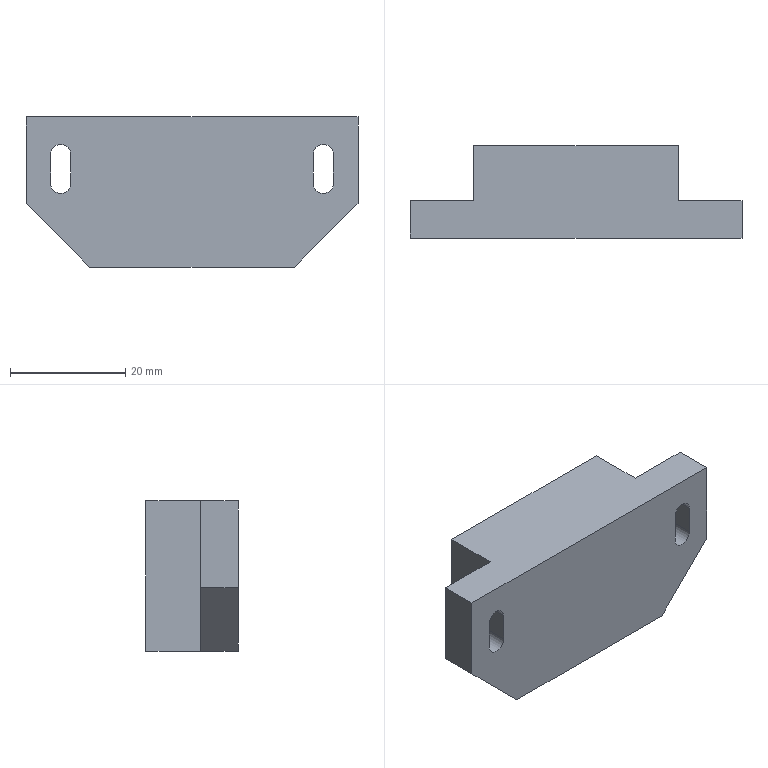Part | STEP file | Large white magnetic mount | 1 solid | 20 faces | box 57.5 x 16 x 26 mm | volume 17347 mm3 | plane 16 | cylinder 4 | commonest cylinder face diameters 3.5 x4
STEP:
#1=CARTESIAN_POINT('',(4.25,6.5,-6.5));
#2=VERTEX_POINT('',#1);
#3=CARTESIAN_POINT('',(7.75,6.5,-6.5));
#4=VERTEX_POINT('',#3);
#5=CARTESIAN_POINT('',(6.,6.5,-6.5));
#6=DIRECTION('',(0.,1.,0.));
#7=DIRECTION('',(0.,0.,1.));
#8=AXIS2_PLACEMENT_3D('',#5,#6,#7);
#9=CIRCLE('',#8,1.75);
#10=EDGE_CURVE('',#2,#4,#9,.T.);
#11=ORIENTED_EDGE('',*,*,#10,.F.);
#12=CARTESIAN_POINT('',(4.25,6.5,-11.5));
#13=VERTEX_POINT('',#12);
#14=CARTESIAN_POINT('',(4.25,6.5,-6.5));
#15=DIRECTION('',(0.,0.,1.));
#16=VECTOR('',#15,1000.);
#17=LINE('',#14,#16);
#18=EDGE_CURVE('',#13,#2,#17,.T.);
#19=ORIENTED_EDGE('',*,*,#18,.F.);
#20=CARTESIAN_POINT('',(7.75,6.5,-11.5));
#21=VERTEX_POINT('',#20);
#22=CARTESIAN_POINT('',(6.,6.5,-11.5));
#23=DIRECTION('',(0.,1.,0.));
#24=DIRECTION('',(0.,0.,1.));
#25=AXIS2_PLACEMENT_3D('',#22,#23,#24);
#26=CIRCLE('',#25,1.75);
#27=EDGE_CURVE('',#21,#13,#26,.T.);
#28=ORIENTED_EDGE('',*,*,#27,.F.);
#29=CARTESIAN_POINT('',(7.75,6.5,-6.5));
#30=DIRECTION('',(0.,0.,-1.));
#31=VECTOR('',#30,1000.);
#32=LINE('',#29,#31);
#33=EDGE_CURVE('',#4,#21,#32,.T.);
#34=ORIENTED_EDGE('',*,*,#33,.F.);
#35=EDGE_LOOP('',(#11,#19,#28,#34));
#36=FACE_BOUND('',#35,.T.);
#37=CARTESIAN_POINT('',(11.,6.5,-26.));
#38=VERTEX_POINT('',#37);
#39=CARTESIAN_POINT('',(11.,6.5,0.));
#40=VERTEX_POINT('',#39);
#41=CARTESIAN_POINT('',(11.,6.5,-26.));
#42=DIRECTION('',(0.,0.,1.));
#43=VECTOR('',#42,1000.);
#44=LINE('',#41,#43);
#45=EDGE_CURVE('',#38,#40,#44,.T.);
#46=ORIENTED_EDGE('',*,*,#45,.F.);
#47=CARTESIAN_POINT('',(0.,6.5,-15.));
#48=VERTEX_POINT('',#47);
#49=CARTESIAN_POINT('',(0.,6.5,-15.));
#50=DIRECTION('',(-0.7071,0.,0.7071));
#51=VECTOR('',#50,1000.);
#52=LINE('',#49,#51);
#53=EDGE_CURVE('',#38,#48,#52,.T.);
#54=ORIENTED_EDGE('',*,*,#53,.T.);
#55=CARTESIAN_POINT('',(0.,6.5,0.));
#56=VERTEX_POINT('',#55);
#57=CARTESIAN_POINT('',(0.,6.5,0.));
#58=DIRECTION('',(0.,0.,1.));
#59=VECTOR('',#58,1000.);
#60=LINE('',#57,#59);
#61=EDGE_CURVE('',#48,#56,#60,.T.);
#62=ORIENTED_EDGE('',*,*,#61,.T.);
#63=CARTESIAN_POINT('',(57.5,6.5,0.));
#64=DIRECTION('',(1.,0.,0.));
#65=VECTOR('',#64,1000.);
#66=LINE('',#63,#65);
#67=EDGE_CURVE('',#56,#40,#66,.T.);
#68=ORIENTED_EDGE('',*,*,#67,.T.);
#69=EDGE_LOOP('',(#46,#54,#62,#68));
#70=FACE_OUTER_BOUND('',#69,.T.);
#71=CARTESIAN_POINT('',(0.,6.5,0.));
#72=DIRECTION('',(0.,-1.,0.));
#73=DIRECTION('',(0.,0.,-1.));
#74=AXIS2_PLACEMENT_3D('',#71,#72,#73);
#75=PLANE('',#74);
#76=ADVANCED_FACE('',(#36,#70),#75,.F.);
#77=CARTESIAN_POINT('',(49.75,6.5,-6.5));
#78=VERTEX_POINT('',#77);
#79=CARTESIAN_POINT('',(53.25,6.5,-6.5));
#80=VERTEX_POINT('',#79);
#81=CARTESIAN_POINT('',(51.5,6.5,-6.5));
#82=DIRECTION('',(0.,1.,0.));
#83=DIRECTION('',(0.,0.,-1.));
#84=AXIS2_PLACEMENT_3D('',#81,#82,#83);
#85=CIRCLE('',#84,1.75);
#86=EDGE_CURVE('',#78,#80,#85,.T.);
#87=ORIENTED_EDGE('',*,*,#86,.F.);
#88=CARTESIAN_POINT('',(49.75,6.5,-11.5));
#89=VERTEX_POINT('',#88);
#90=CARTESIAN_POINT('',(49.75,6.5,-6.5));
#91=DIRECTION('',(0.,0.,1.));
#92=VECTOR('',#91,1000.);
#93=LINE('',#90,#92);
#94=EDGE_CURVE('',#89,#78,#93,.T.);
#95=ORIENTED_EDGE('',*,*,#94,.F.);
#96=CARTESIAN_POINT('',(53.25,6.5,-11.5));
#97=VERTEX_POINT('',#96);
#98=CARTESIAN_POINT('',(51.5,6.5,-11.5));
#99=DIRECTION('',(0.,1.,0.));
#100=DIRECTION('',(0.,0.,-1.));
#101=AXIS2_PLACEMENT_3D('',#98,#99,#100);
#102=CIRCLE('',#101,1.75);
#103=EDGE_CURVE('',#97,#89,#102,.T.);
#104=ORIENTED_EDGE('',*,*,#103,.F.);
#105=CARTESIAN_POINT('',(53.25,6.5,-6.5));
#106=DIRECTION('',(0.,0.,-1.));
#107=VECTOR('',#106,1000.);
#108=LINE('',#105,#107);
#109=EDGE_CURVE('',#80,#97,#108,.T.);
#110=ORIENTED_EDGE('',*,*,#109,.F.);
#111=EDGE_LOOP('',(#87,#95,#104,#110));
#112=FACE_BOUND('',#111,.T.);
#113=CARTESIAN_POINT('',(46.5,6.5,0.));
#114=VERTEX_POINT('',#113);
#115=CARTESIAN_POINT('',(46.5,6.5,-26.));
#116=VERTEX_POINT('',#115);
#117=CARTESIAN_POINT('',(46.5,6.5,-26.));
#118=DIRECTION('',(0.,0.,-1.));
#119=VECTOR('',#118,1000.);
#120=LINE('',#117,#119);
#121=EDGE_CURVE('',#114,#116,#120,.T.);
#122=ORIENTED_EDGE('',*,*,#121,.F.);
#123=CARTESIAN_POINT('',(57.5,6.5,0.));
#124=VERTEX_POINT('',#123);
#125=CARTESIAN_POINT('',(57.5,6.5,0.));
#126=DIRECTION('',(1.,0.,0.));
#127=VECTOR('',#126,1000.);
#128=LINE('',#125,#127);
#129=EDGE_CURVE('',#114,#124,#128,.T.);
#130=ORIENTED_EDGE('',*,*,#129,.T.);
#131=CARTESIAN_POINT('',(57.5,6.5,-15.));
#132=VERTEX_POINT('',#131);
#133=CARTESIAN_POINT('',(57.5,6.5,-15.));
#134=DIRECTION('',(0.,0.,-1.));
#135=VECTOR('',#134,1000.);
#136=LINE('',#133,#135);
#137=EDGE_CURVE('',#124,#132,#136,.T.);
#138=ORIENTED_EDGE('',*,*,#137,.T.);
#139=CARTESIAN_POINT('',(46.5,6.5,-26.));
#140=DIRECTION('',(-0.7071,0.,-0.7071));
#141=VECTOR('',#140,1000.);
#142=LINE('',#139,#141);
#143=EDGE_CURVE('',#132,#116,#142,.T.);
#144=ORIENTED_EDGE('',*,*,#143,.T.);
#145=EDGE_LOOP('',(#122,#130,#138,#144));
#146=FACE_OUTER_BOUND('',#145,.T.);
#147=CARTESIAN_POINT('',(0.,6.5,0.));
#148=DIRECTION('',(0.,-1.,0.));
#149=DIRECTION('',(0.,0.,-1.));
#150=AXIS2_PLACEMENT_3D('',#147,#148,#149);
#151=PLANE('',#150);
#152=ADVANCED_FACE('',(#112,#146),#151,.F.);
#153=CARTESIAN_POINT('',(0.,0.,0.));
#154=VERTEX_POINT('',#153);
#155=CARTESIAN_POINT('',(57.5,0.,0.));
#156=VERTEX_POINT('',#155);
#157=CARTESIAN_POINT('',(57.5,0.,0.));
#158=DIRECTION('',(1.,0.,0.));
#159=VECTOR('',#158,1000.);
#160=LINE('',#157,#159);
#161=EDGE_CURVE('',#154,#156,#160,.T.);
#162=ORIENTED_EDGE('',*,*,#161,.F.);
#163=CARTESIAN_POINT('',(0.,0.,-15.));
#164=VERTEX_POINT('',#163);
#165=CARTESIAN_POINT('',(0.,0.,0.));
#166=DIRECTION('',(0.,0.,1.));
#167=VECTOR('',#166,1000.);
#168=LINE('',#165,#167);
#169=EDGE_CURVE('',#164,#154,#168,.T.);
#170=ORIENTED_EDGE('',*,*,#169,.F.);
#171=CARTESIAN_POINT('',(11.,0.,-26.));
#172=VERTEX_POINT('',#171);
#173=CARTESIAN_POINT('',(0.,0.,-15.));
#174=DIRECTION('',(-0.7071,0.,0.7071));
#175=VECTOR('',#174,1000.);
#176=LINE('',#173,#175);
#177=EDGE_CURVE('',#172,#164,#176,.T.);
#178=ORIENTED_EDGE('',*,*,#177,.F.);
#179=CARTESIAN_POINT('',(46.5,0.,-26.));
#180=VERTEX_POINT('',#179);
#181=CARTESIAN_POINT('',(11.,0.,-26.));
#182=DIRECTION('',(-1.,0.,0.));
#183=VECTOR('',#182,1000.);
#184=LINE('',#181,#183);
#185=EDGE_CURVE('',#180,#172,#184,.T.);
#186=ORIENTED_EDGE('',*,*,#185,.F.);
#187=CARTESIAN_POINT('',(57.5,0.,-15.));
#188=VERTEX_POINT('',#187);
#189=CARTESIAN_POINT('',(46.5,0.,-26.));
#190=DIRECTION('',(-0.7071,0.,-0.7071));
#191=VECTOR('',#190,1000.);
#192=LINE('',#189,#191);
#193=EDGE_CURVE('',#188,#180,#192,.T.);
#194=ORIENTED_EDGE('',*,*,#193,.F.);
#195=CARTESIAN_POINT('',(57.5,0.,-15.));
#196=DIRECTION('',(0.,0.,-1.));
#197=VECTOR('',#196,1000.);
#198=LINE('',#195,#197);
#199=EDGE_CURVE('',#156,#188,#198,.T.);
#200=ORIENTED_EDGE('',*,*,#199,.F.);
#201=EDGE_LOOP('',(#162,#170,#178,#186,#194,#200));
#202=FACE_OUTER_BOUND('',#201,.T.);
#203=CARTESIAN_POINT('',(4.25,0.,-11.5));
#204=VERTEX_POINT('',#203);
#205=CARTESIAN_POINT('',(4.25,0.,-6.5));
#206=VERTEX_POINT('',#205);
#207=CARTESIAN_POINT('',(4.25,0.,-6.5));
#208=DIRECTION('',(0.,0.,1.));
#209=VECTOR('',#208,1000.);
#210=LINE('',#207,#209);
#211=EDGE_CURVE('',#204,#206,#210,.T.);
#212=ORIENTED_EDGE('',*,*,#211,.T.);
#213=CARTESIAN_POINT('',(7.75,0.,-6.5));
#214=VERTEX_POINT('',#213);
#215=CARTESIAN_POINT('',(6.,0.,-6.5));
#216=DIRECTION('',(0.,1.,0.));
#217=DIRECTION('',(0.,0.,1.));
#218=AXIS2_PLACEMENT_3D('',#215,#216,#217);
#219=CIRCLE('',#218,1.75);
#220=EDGE_CURVE('',#206,#214,#219,.T.);
#221=ORIENTED_EDGE('',*,*,#220,.T.);
#222=CARTESIAN_POINT('',(7.75,0.,-11.5));
#223=VERTEX_POINT('',#222);
#224=CARTESIAN_POINT('',(7.75,0.,-6.5));
#225=DIRECTION('',(0.,0.,-1.));
#226=VECTOR('',#225,1000.);
#227=LINE('',#224,#226);
#228=EDGE_CURVE('',#214,#223,#227,.T.);
#229=ORIENTED_EDGE('',*,*,#228,.T.);
#230=CARTESIAN_POINT('',(6.,0.,-11.5));
#231=DIRECTION('',(0.,1.,0.));
#232=DIRECTION('',(0.,0.,1.));
#233=AXIS2_PLACEMENT_3D('',#230,#231,#232);
#234=CIRCLE('',#233,1.75);
#235=EDGE_CURVE('',#223,#204,#234,.T.);
#236=ORIENTED_EDGE('',*,*,#235,.T.);
#237=EDGE_LOOP('',(#212,#221,#229,#236));
#238=FACE_BOUND('',#237,.T.);
#239=CARTESIAN_POINT('',(49.75,0.,-11.5));
#240=VERTEX_POINT('',#239);
#241=CARTESIAN_POINT('',(49.75,0.,-6.5));
#242=VERTEX_POINT('',#241);
#243=CARTESIAN_POINT('',(49.75,0.,-6.5));
#244=DIRECTION('',(0.,0.,1.));
#245=VECTOR('',#244,1000.);
#246=LINE('',#243,#245);
#247=EDGE_CURVE('',#240,#242,#246,.T.);
#248=ORIENTED_EDGE('',*,*,#247,.T.);
#249=CARTESIAN_POINT('',(53.25,0.,-6.5));
#250=VERTEX_POINT('',#249);
#251=CARTESIAN_POINT('',(51.5,0.,-6.5));
#252=DIRECTION('',(0.,1.,0.));
#253=DIRECTION('',(0.,0.,-1.));
#254=AXIS2_PLACEMENT_3D('',#251,#252,#253);
#255=CIRCLE('',#254,1.75);
#256=EDGE_CURVE('',#242,#250,#255,.T.);
#257=ORIENTED_EDGE('',*,*,#256,.T.);
#258=CARTESIAN_POINT('',(53.25,0.,-11.5));
#259=VERTEX_POINT('',#258);
#260=CARTESIAN_POINT('',(53.25,0.,-6.5));
#261=DIRECTION('',(0.,0.,-1.));
#262=VECTOR('',#261,1000.);
#263=LINE('',#260,#262);
#264=EDGE_CURVE('',#250,#259,#263,.T.);
#265=ORIENTED_EDGE('',*,*,#264,.T.);
#266=CARTESIAN_POINT('',(51.5,0.,-11.5));
#267=DIRECTION('',(0.,1.,0.));
#268=DIRECTION('',(0.,0.,-1.));
#269=AXIS2_PLACEMENT_3D('',#266,#267,#268);
#270=CIRCLE('',#269,1.75);
#271=EDGE_CURVE('',#259,#240,#270,.T.);
#272=ORIENTED_EDGE('',*,*,#271,.T.);
#273=EDGE_LOOP('',(#248,#257,#265,#272));
#274=FACE_BOUND('',#273,.T.);
#275=CARTESIAN_POINT('',(0.,0.,0.));
#276=DIRECTION('',(0.,-1.,0.));
#277=DIRECTION('',(0.,0.,-1.));
#278=AXIS2_PLACEMENT_3D('',#275,#276,#277);
#279=PLANE('',#278);
#280=ADVANCED_FACE('',(#202,#238,#274),#279,.T.);
#281=ORIENTED_EDGE('',*,*,#161,.T.);
#282=CARTESIAN_POINT('',(57.5,6.5,0.));
#283=DIRECTION('',(0.,-1.,0.));
#284=VECTOR('',#283,1000.);
#285=LINE('',#282,#284);
#286=EDGE_CURVE('',#124,#156,#285,.T.);
#287=ORIENTED_EDGE('',*,*,#286,.F.);
#288=ORIENTED_EDGE('',*,*,#129,.F.);
#289=CARTESIAN_POINT('',(46.5,16.,0.));
#290=VERTEX_POINT('',#289);
#291=CARTESIAN_POINT('',(46.5,16.,0.));
#292=DIRECTION('',(0.,-1.,0.));
#293=VECTOR('',#292,1000.);
#294=LINE('',#291,#293);
#295=EDGE_CURVE('',#290,#114,#294,.T.);
#296=ORIENTED_EDGE('',*,*,#295,.F.);
#297=CARTESIAN_POINT('',(11.,16.,0.));
#298=VERTEX_POINT('',#297);
#299=CARTESIAN_POINT('',(11.,16.,0.));
#300=DIRECTION('',(1.,0.,0.));
#301=VECTOR('',#300,1000.);
#302=LINE('',#299,#301);
#303=EDGE_CURVE('',#298,#290,#302,.T.);
#304=ORIENTED_EDGE('',*,*,#303,.F.);
#305=CARTESIAN_POINT('',(11.,16.,0.));
#306=DIRECTION('',(0.,-1.,0.));
#307=VECTOR('',#306,1000.);
#308=LINE('',#305,#307);
#309=EDGE_CURVE('',#298,#40,#308,.T.);
#310=ORIENTED_EDGE('',*,*,#309,.T.);
#311=ORIENTED_EDGE('',*,*,#67,.F.);
#312=CARTESIAN_POINT('',(0.,6.5,0.));
#313=DIRECTION('',(0.,-1.,0.));
#314=VECTOR('',#313,1000.);
#315=LINE('',#312,#314);
#316=EDGE_CURVE('',#56,#154,#315,.T.);
#317=ORIENTED_EDGE('',*,*,#316,.T.);
#318=EDGE_LOOP('',(#281,#287,#288,#296,#304,#310,#311,#317));
#319=FACE_OUTER_BOUND('',#318,.T.);
#320=CARTESIAN_POINT('',(57.5,6.5,0.));
#321=DIRECTION('',(0.,0.,-1.));
#322=DIRECTION('',(-1.,0.,0.));
#323=AXIS2_PLACEMENT_3D('',#320,#321,#322);
#324=PLANE('',#323);
#325=ADVANCED_FACE('',(#319),#324,.F.);
#326=ORIENTED_EDGE('',*,*,#199,.T.);
#327=CARTESIAN_POINT('',(57.5,6.5,-15.));
#328=DIRECTION('',(0.,-1.,0.));
#329=VECTOR('',#328,1000.);
#330=LINE('',#327,#329);
#331=EDGE_CURVE('',#132,#188,#330,.T.);
#332=ORIENTED_EDGE('',*,*,#331,.F.);
#333=ORIENTED_EDGE('',*,*,#137,.F.);
#334=ORIENTED_EDGE('',*,*,#286,.T.);
#335=EDGE_LOOP('',(#326,#332,#333,#334));
#336=FACE_OUTER_BOUND('',#335,.T.);
#337=CARTESIAN_POINT('',(57.5,6.5,-15.));
#338=DIRECTION('',(-1.,0.,0.));
#339=DIRECTION('',(0.,0.,1.));
#340=AXIS2_PLACEMENT_3D('',#337,#338,#339);
#341=PLANE('',#340);
#342=ADVANCED_FACE('',(#336),#341,.F.);
#343=ORIENTED_EDGE('',*,*,#193,.T.);
#344=CARTESIAN_POINT('',(46.5,6.5,-26.));
#345=DIRECTION('',(0.,-1.,0.));
#346=VECTOR('',#345,1000.);
#347=LINE('',#344,#346);
#348=EDGE_CURVE('',#116,#180,#347,.T.);
#349=ORIENTED_EDGE('',*,*,#348,.F.);
#350=ORIENTED_EDGE('',*,*,#143,.F.);
#351=ORIENTED_EDGE('',*,*,#331,.T.);
#352=EDGE_LOOP('',(#343,#349,#350,#351));
#353=FACE_OUTER_BOUND('',#352,.T.);
#354=CARTESIAN_POINT('',(46.5,6.5,-26.));
#355=DIRECTION('',(-0.7071,0.,0.7071));
#356=DIRECTION('',(0.7071,0.,0.7071));
#357=AXIS2_PLACEMENT_3D('',#354,#355,#356);
#358=PLANE('',#357);
#359=ADVANCED_FACE('',(#353),#358,.F.);
#360=ORIENTED_EDGE('',*,*,#185,.T.);
#361=CARTESIAN_POINT('',(11.,6.5,-26.));
#362=DIRECTION('',(0.,-1.,0.));
#363=VECTOR('',#362,1000.);
#364=LINE('',#361,#363);
#365=EDGE_CURVE('',#38,#172,#364,.T.);
#366=ORIENTED_EDGE('',*,*,#365,.F.);
#367=CARTESIAN_POINT('',(11.,16.,-26.));
#368=VERTEX_POINT('',#367);
#369=CARTESIAN_POINT('',(11.,16.,-26.));
#370=DIRECTION('',(0.,-1.,0.));
#371=VECTOR('',#370,1000.);
#372=LINE('',#369,#371);
#373=EDGE_CURVE('',#368,#38,#372,.T.);
#374=ORIENTED_EDGE('',*,*,#373,.F.);
#375=CARTESIAN_POINT('',(46.5,16.,-26.));
#376=VERTEX_POINT('',#375);
#377=CARTESIAN_POINT('',(11.,16.,-26.));
#378=DIRECTION('',(-1.,0.,0.));
#379=VECTOR('',#378,1000.);
#380=LINE('',#377,#379);
#381=EDGE_CURVE('',#376,#368,#380,.T.);
#382=ORIENTED_EDGE('',*,*,#381,.F.);
#383=CARTESIAN_POINT('',(46.5,16.,-26.));
#384=DIRECTION('',(0.,-1.,0.));
#385=VECTOR('',#384,1000.);
#386=LINE('',#383,#385);
#387=EDGE_CURVE('',#376,#116,#386,.T.);
#388=ORIENTED_EDGE('',*,*,#387,.T.);
#389=ORIENTED_EDGE('',*,*,#348,.T.);
#390=EDGE_LOOP('',(#360,#366,#374,#382,#388,#389));
#391=FACE_OUTER_BOUND('',#390,.T.);
#392=CARTESIAN_POINT('',(11.,6.5,-26.));
#393=DIRECTION('',(0.,0.,1.));
#394=DIRECTION('',(1.,0.,0.));
#395=AXIS2_PLACEMENT_3D('',#392,#393,#394);
#396=PLANE('',#395);
#397=ADVANCED_FACE('',(#391),#396,.F.);
#398=ORIENTED_EDGE('',*,*,#177,.T.);
#399=CARTESIAN_POINT('',(0.,6.5,-15.));
#400=DIRECTION('',(0.,-1.,0.));
#401=VECTOR('',#400,1000.);
#402=LINE('',#399,#401);
#403=EDGE_CURVE('',#48,#164,#402,.T.);
#404=ORIENTED_EDGE('',*,*,#403,.F.);
#405=ORIENTED_EDGE('',*,*,#53,.F.);
#406=ORIENTED_EDGE('',*,*,#365,.T.);
#407=EDGE_LOOP('',(#398,#404,#405,#406));
#408=FACE_OUTER_BOUND('',#407,.T.);
#409=CARTESIAN_POINT('',(0.,6.5,-15.));
#410=DIRECTION('',(0.7071,0.,0.7071));
#411=DIRECTION('',(0.7071,0.,-0.7071));
#412=AXIS2_PLACEMENT_3D('',#409,#410,#411);
#413=PLANE('',#412);
#414=ADVANCED_FACE('',(#408),#413,.F.);
#415=ORIENTED_EDGE('',*,*,#169,.T.);
#416=ORIENTED_EDGE('',*,*,#316,.F.);
#417=ORIENTED_EDGE('',*,*,#61,.F.);
#418=ORIENTED_EDGE('',*,*,#403,.T.);
#419=EDGE_LOOP('',(#415,#416,#417,#418));
#420=FACE_OUTER_BOUND('',#419,.T.);
#421=CARTESIAN_POINT('',(0.,6.5,0.));
#422=DIRECTION('',(1.,0.,0.));
#423=DIRECTION('',(0.,0.,-1.));
#424=AXIS2_PLACEMENT_3D('',#421,#422,#423);
#425=PLANE('',#424);
#426=ADVANCED_FACE('',(#420),#425,.F.);
#427=ORIENTED_EDGE('',*,*,#220,.F.);
#428=CARTESIAN_POINT('',(4.25,6.5,-6.5));
#429=DIRECTION('',(0.,-1.,0.));
#430=VECTOR('',#429,1000.);
#431=LINE('',#428,#430);
#432=EDGE_CURVE('',#2,#206,#431,.T.);
#433=ORIENTED_EDGE('',*,*,#432,.F.);
#434=ORIENTED_EDGE('',*,*,#10,.T.);
#435=CARTESIAN_POINT('',(7.75,6.5,-6.5));
#436=DIRECTION('',(0.,-1.,0.));
#437=VECTOR('',#436,1000.);
#438=LINE('',#435,#437);
#439=EDGE_CURVE('',#4,#214,#438,.T.);
#440=ORIENTED_EDGE('',*,*,#439,.T.);
#441=EDGE_LOOP('',(#427,#433,#434,#440));
#442=FACE_OUTER_BOUND('',#441,.T.);
#443=CARTESIAN_POINT('',(6.,6.5,-6.5));
#444=DIRECTION('',(0.,-1.,0.));
#445=DIRECTION('',(0.,0.,-1.));
#446=AXIS2_PLACEMENT_3D('',#443,#444,#445);
#447=CYLINDRICAL_SURFACE('',#446,1.75);
#448=ADVANCED_FACE('',(#442),#447,.F.);
#449=ORIENTED_EDGE('',*,*,#228,.F.);
#450=ORIENTED_EDGE('',*,*,#439,.F.);
#451=ORIENTED_EDGE('',*,*,#33,.T.);
#452=CARTESIAN_POINT('',(7.75,6.5,-11.5));
#453=DIRECTION('',(0.,-1.,0.));
#454=VECTOR('',#453,1000.);
#455=LINE('',#452,#454);
#456=EDGE_CURVE('',#21,#223,#455,.T.);
#457=ORIENTED_EDGE('',*,*,#456,.T.);
#458=EDGE_LOOP('',(#449,#450,#451,#457));
#459=FACE_OUTER_BOUND('',#458,.T.);
#460=CARTESIAN_POINT('',(7.75,6.5,-6.5));
#461=DIRECTION('',(-1.,0.,0.));
#462=DIRECTION('',(0.,0.,1.));
#463=AXIS2_PLACEMENT_3D('',#460,#461,#462);
#464=PLANE('',#463);
#465=ADVANCED_FACE('',(#459),#464,.T.);
#466=ORIENTED_EDGE('',*,*,#235,.F.);
#467=ORIENTED_EDGE('',*,*,#456,.F.);
#468=ORIENTED_EDGE('',*,*,#27,.T.);
#469=CARTESIAN_POINT('',(4.25,6.5,-11.5));
#470=DIRECTION('',(0.,-1.,0.));
#471=VECTOR('',#470,1000.);
#472=LINE('',#469,#471);
#473=EDGE_CURVE('',#13,#204,#472,.T.);
#474=ORIENTED_EDGE('',*,*,#473,.T.);
#475=EDGE_LOOP('',(#466,#467,#468,#474));
#476=FACE_OUTER_BOUND('',#475,.T.);
#477=CARTESIAN_POINT('',(6.,6.5,-11.5));
#478=DIRECTION('',(0.,-1.,0.));
#479=DIRECTION('',(0.,0.,-1.));
#480=AXIS2_PLACEMENT_3D('',#477,#478,#479);
#481=CYLINDRICAL_SURFACE('',#480,1.75);
#482=ADVANCED_FACE('',(#476),#481,.F.);
#483=ORIENTED_EDGE('',*,*,#211,.F.);
#484=ORIENTED_EDGE('',*,*,#473,.F.);
#485=ORIENTED_EDGE('',*,*,#18,.T.);
#486=ORIENTED_EDGE('',*,*,#432,.T.);
#487=EDGE_LOOP('',(#483,#484,#485,#486));
#488=FACE_OUTER_BOUND('',#487,.T.);
#489=CARTESIAN_POINT('',(4.25,6.5,-6.5));
#490=DIRECTION('',(1.,0.,0.));
#491=DIRECTION('',(0.,0.,-1.));
#492=AXIS2_PLACEMENT_3D('',#489,#490,#491);
#493=PLANE('',#492);
#494=ADVANCED_FACE('',(#488),#493,.T.);
#495=ORIENTED_EDGE('',*,*,#256,.F.);
#496=CARTESIAN_POINT('',(49.75,6.5,-6.5));
#497=DIRECTION('',(0.,-1.,0.));
#498=VECTOR('',#497,1000.);
#499=LINE('',#496,#498);
#500=EDGE_CURVE('',#78,#242,#499,.T.);
#501=ORIENTED_EDGE('',*,*,#500,.F.);
#502=ORIENTED_EDGE('',*,*,#86,.T.);
#503=CARTESIAN_POINT('',(53.25,6.5,-6.5));
#504=DIRECTION('',(0.,-1.,0.));
#505=VECTOR('',#504,1000.);
#506=LINE('',#503,#505);
#507=EDGE_CURVE('',#80,#250,#506,.T.);
#508=ORIENTED_EDGE('',*,*,#507,.T.);
#509=EDGE_LOOP('',(#495,#501,#502,#508));
#510=FACE_OUTER_BOUND('',#509,.T.);
#511=CARTESIAN_POINT('',(51.5,6.5,-6.5));
#512=DIRECTION('',(0.,-1.,0.));
#513=DIRECTION('',(0.,0.,-1.));
#514=AXIS2_PLACEMENT_3D('',#511,#512,#513);
#515=CYLINDRICAL_SURFACE('',#514,1.75);
#516=ADVANCED_FACE('',(#510),#515,.F.);
#517=ORIENTED_EDGE('',*,*,#264,.F.);
#518=ORIENTED_EDGE('',*,*,#507,.F.);
#519=ORIENTED_EDGE('',*,*,#109,.T.);
#520=CARTESIAN_POINT('',(53.25,6.5,-11.5));
#521=DIRECTION('',(0.,-1.,0.));
#522=VECTOR('',#521,1000.);
#523=LINE('',#520,#522);
#524=EDGE_CURVE('',#97,#259,#523,.T.);
#525=ORIENTED_EDGE('',*,*,#524,.T.);
#526=EDGE_LOOP('',(#517,#518,#519,#525));
#527=FACE_OUTER_BOUND('',#526,.T.);
#528=CARTESIAN_POINT('',(53.25,6.5,-6.5));
#529=DIRECTION('',(-1.,0.,0.));
#530=DIRECTION('',(0.,0.,1.));
#531=AXIS2_PLACEMENT_3D('',#528,#529,#530);
#532=PLANE('',#531);
#533=ADVANCED_FACE('',(#527),#532,.T.);
#534=ORIENTED_EDGE('',*,*,#271,.F.);
#535=ORIENTED_EDGE('',*,*,#524,.F.);
#536=ORIENTED_EDGE('',*,*,#103,.T.);
#537=CARTESIAN_POINT('',(49.75,6.5,-11.5));
#538=DIRECTION('',(0.,-1.,0.));
#539=VECTOR('',#538,1000.);
#540=LINE('',#537,#539);
#541=EDGE_CURVE('',#89,#240,#540,.T.);
#542=ORIENTED_EDGE('',*,*,#541,.T.);
#543=EDGE_LOOP('',(#534,#535,#536,#542));
#544=FACE_OUTER_BOUND('',#543,.T.);
#545=CARTESIAN_POINT('',(51.5,6.5,-11.5));
#546=DIRECTION('',(0.,-1.,0.));
#547=DIRECTION('',(0.,0.,-1.));
#548=AXIS2_PLACEMENT_3D('',#545,#546,#547);
#549=CYLINDRICAL_SURFACE('',#548,1.75);
#550=ADVANCED_FACE('',(#544),#549,.F.);
#551=ORIENTED_EDGE('',*,*,#247,.F.);
#552=ORIENTED_EDGE('',*,*,#541,.F.);
#553=ORIENTED_EDGE('',*,*,#94,.T.);
#554=ORIENTED_EDGE('',*,*,#500,.T.);
#555=EDGE_LOOP('',(#551,#552,#553,#554));
#556=FACE_OUTER_BOUND('',#555,.T.);
#557=CARTESIAN_POINT('',(49.75,6.5,-6.5));
#558=DIRECTION('',(1.,0.,0.));
#559=DIRECTION('',(0.,0.,-1.));
#560=AXIS2_PLACEMENT_3D('',#557,#558,#559);
#561=PLANE('',#560);
#562=ADVANCED_FACE('',(#556),#561,.T.);
#563=ORIENTED_EDGE('',*,*,#45,.T.);
#564=ORIENTED_EDGE('',*,*,#309,.F.);
#565=CARTESIAN_POINT('',(11.,16.,-26.));
#566=DIRECTION('',(0.,0.,1.));
#567=VECTOR('',#566,1000.);
#568=LINE('',#565,#567);
#569=EDGE_CURVE('',#368,#298,#568,.T.);
#570=ORIENTED_EDGE('',*,*,#569,.F.);
#571=ORIENTED_EDGE('',*,*,#373,.T.);
#572=EDGE_LOOP('',(#563,#564,#570,#571));
#573=FACE_OUTER_BOUND('',#572,.T.);
#574=CARTESIAN_POINT('',(11.,16.,-26.));
#575=DIRECTION('',(1.,0.,0.));
#576=DIRECTION('',(0.,0.,-1.));
#577=AXIS2_PLACEMENT_3D('',#574,#575,#576);
#578=PLANE('',#577);
#579=ADVANCED_FACE('',(#573),#578,.F.);
#580=ORIENTED_EDGE('',*,*,#121,.T.);
#581=ORIENTED_EDGE('',*,*,#387,.F.);
#582=CARTESIAN_POINT('',(46.5,16.,-26.));
#583=DIRECTION('',(0.,0.,-1.));
#584=VECTOR('',#583,1000.);
#585=LINE('',#582,#584);
#586=EDGE_CURVE('',#290,#376,#585,.T.);
#587=ORIENTED_EDGE('',*,*,#586,.F.);
#588=ORIENTED_EDGE('',*,*,#295,.T.);
#589=EDGE_LOOP('',(#580,#581,#587,#588));
#590=FACE_OUTER_BOUND('',#589,.T.);
#591=CARTESIAN_POINT('',(46.5,16.,-26.));
#592=DIRECTION('',(-1.,0.,0.));
#593=DIRECTION('',(0.,0.,1.));
#594=AXIS2_PLACEMENT_3D('',#591,#592,#593);
#595=PLANE('',#594);
#596=ADVANCED_FACE('',(#590),#595,.F.);
#597=ORIENTED_EDGE('',*,*,#569,.T.);
#598=ORIENTED_EDGE('',*,*,#303,.T.);
#599=ORIENTED_EDGE('',*,*,#586,.T.);
#600=ORIENTED_EDGE('',*,*,#381,.T.);
#601=EDGE_LOOP('',(#597,#598,#599,#600));
#602=FACE_OUTER_BOUND('',#601,.T.);
#603=CARTESIAN_POINT('',(0.,16.,0.));
#604=DIRECTION('',(0.,1.,0.));
#605=DIRECTION('',(0.,0.,1.));
#606=AXIS2_PLACEMENT_3D('',#603,#604,#605);
#607=PLANE('',#606);
#608=ADVANCED_FACE('',(#602),#607,.T.);
#609=CLOSED_SHELL('',(#76,#152,#280,#325,#342,#359,#397,#414,#426,#448,#465,#482,#494,#516,#533,#550,#562,#579,#596,#608));
#610=MANIFOLD_SOLID_BREP('',#609);
#611=CARTESIAN_POINT('',(0.,0.,0.));
#612=DIRECTION('',(0.,0.,1.));
#613=DIRECTION('',(1.,0.,0.));
#614=AXIS2_PLACEMENT_3D('',#611,#612,#613);
#615=(LENGTH_UNIT()NAMED_UNIT(*)SI_UNIT(.MILLI.,.METRE.));
#616=UNCERTAINTY_MEASURE_WITH_UNIT(LENGTH_MEASURE(0.00001),#615,'','');
#617=(NAMED_UNIT(*)PLANE_ANGLE_UNIT()SI_UNIT($,.RADIAN.));
#618=(NAMED_UNIT(*)SI_UNIT($,.STERADIAN.)SOLID_ANGLE_UNIT());
#619=(GEOMETRIC_REPRESENTATION_CONTEXT(3)GLOBAL_UNCERTAINTY_ASSIGNED_CONTEXT((#616))GLOBAL_UNIT_ASSIGNED_CONTEXT((#615,#617,#618))REPRESENTATION_CONTEXT('',''));
#620=ADVANCED_BREP_SHAPE_REPRESENTATION('',(#610,#614),#619);